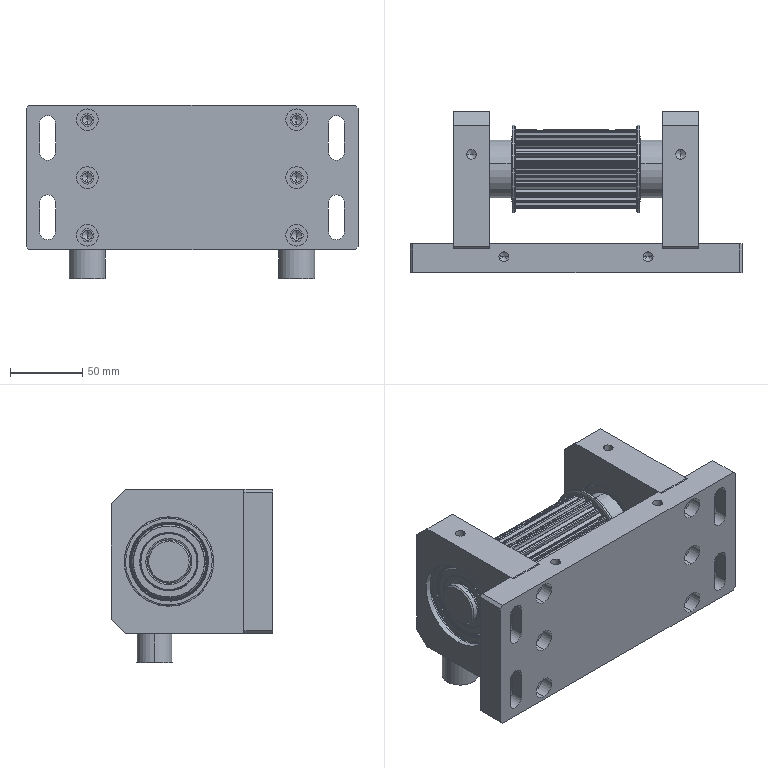Part | SolidWorks | 13 solids | 798 faces | box 230 x 112 x 120 mm | volume 1042878 mm3 | cylinder 427 | cone 136 | plane 131 | spline 104 | commonest cylinder face diameters 0.8 x60 1.5 x60 10.6 x54 48.99 x29 6.8 x24 54.65 x24